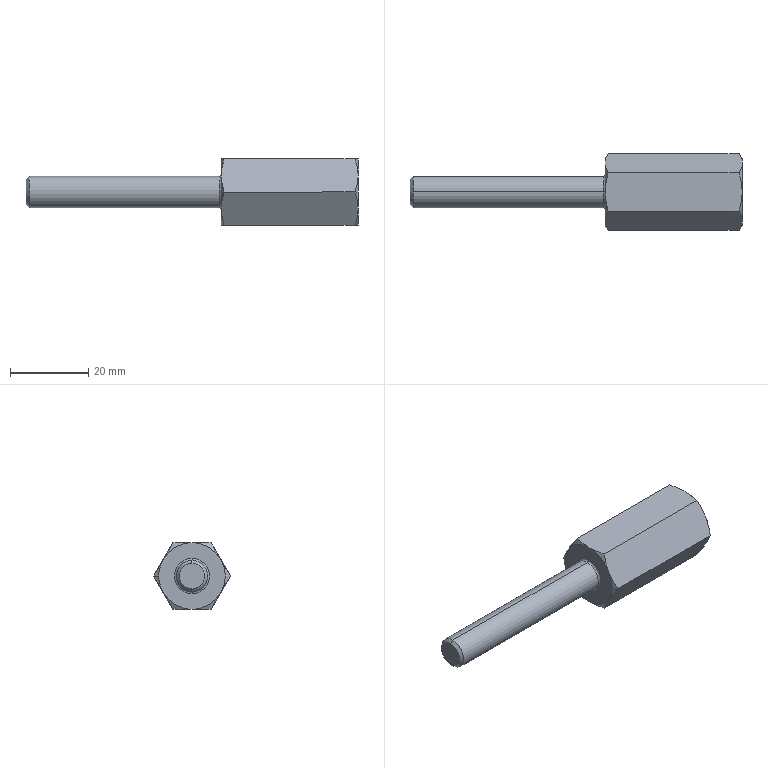Part | STEP file | 0228_005_SLSBH17-35-F50-M8-N6 | 1 solid | 35 faces | box 85 x 19.63 x 17 mm | volume 10911 mm3 | cone 20 | plane 9 | cylinder 4 | torus 2 | commonest cylinder face diameters 5 x2 8 x2